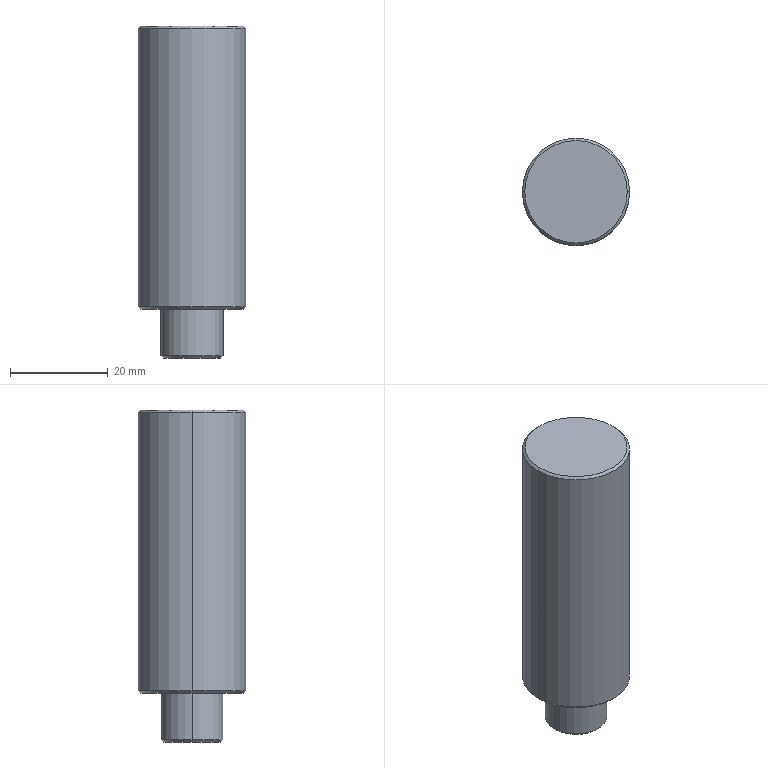Part | SolidWorks | features Chamfer 1, Extrusion 1, ICE 1 | 1 solid | 13 faces | box 22 x 22 x 68 mm | volume 23293 mm3 | cone 6 | cylinder 4 | plane 3 | commonest cylinder face diameters 12.7 x2 22 x2
STEP:
#1=CARTESIAN_POINT('',(-5.85,0.,0.));
#2=VERTEX_POINT('',#1);
#3=CARTESIAN_POINT('',(5.85,0.,0.));
#4=VERTEX_POINT('',#3);
#5=CARTESIAN_POINT('',(0.,0.,0.));
#6=DIRECTION('',(0.,0.,-1.));
#7=DIRECTION('',(1.,0.,0.));
#8=AXIS2_PLACEMENT_3D('',#5,#6,#7);
#9=CIRCLE('',#8,5.85);
#10=EDGE_CURVE('',#2,#4,#9,.T.);
#11=ORIENTED_EDGE('',*,*,#10,.F.);
#12=CARTESIAN_POINT('',(-6.35,0.,0.5));
#13=VERTEX_POINT('',#12);
#14=CARTESIAN_POINT('',(-6.35,0.,0.5));
#15=DIRECTION('',(-0.7071,0.,0.7071));
#16=VECTOR('',#15,1000.);
#17=LINE('',#14,#16);
#18=EDGE_CURVE('',#2,#13,#17,.T.);
#19=ORIENTED_EDGE('',*,*,#18,.T.);
#20=CARTESIAN_POINT('',(6.35,0.,0.5));
#21=VERTEX_POINT('',#20);
#22=CARTESIAN_POINT('',(0.,0.,0.5));
#23=DIRECTION('',(0.,0.,1.));
#24=DIRECTION('',(1.,0.,0.));
#25=AXIS2_PLACEMENT_3D('',#22,#23,#24);
#26=CIRCLE('',#25,6.35);
#27=EDGE_CURVE('',#21,#13,#26,.T.);
#28=ORIENTED_EDGE('',*,*,#27,.F.);
#29=CARTESIAN_POINT('',(6.35,0.,0.5));
#30=DIRECTION('',(0.7071,0.,0.7071));
#31=VECTOR('',#30,1000.);
#32=LINE('',#29,#31);
#33=EDGE_CURVE('',#4,#21,#32,.T.);
#34=ORIENTED_EDGE('',*,*,#33,.F.);
#35=EDGE_LOOP('',(#11,#19,#28,#34));
#36=FACE_OUTER_BOUND('',#35,.T.);
#37=CARTESIAN_POINT('',(0.,0.,0.5));
#38=DIRECTION('',(0.,0.,1.));
#39=DIRECTION('',(1.,0.,0.));
#40=AXIS2_PLACEMENT_3D('',#37,#38,#39);
#41=CONICAL_SURFACE('',#40,6.35,0.7854);
#42=ADVANCED_FACE('',(#36),#41,.T.);
#43=CARTESIAN_POINT('',(10.5,0.,68.));
#44=VERTEX_POINT('',#43);
#45=CARTESIAN_POINT('',(-10.5,0.,68.));
#46=VERTEX_POINT('',#45);
#47=CARTESIAN_POINT('',(0.,0.,68.));
#48=DIRECTION('',(0.,0.,1.));
#49=DIRECTION('',(1.,0.,0.));
#50=AXIS2_PLACEMENT_3D('',#47,#48,#49);
#51=CIRCLE('',#50,10.5);
#52=EDGE_CURVE('',#44,#46,#51,.T.);
#53=ORIENTED_EDGE('',*,*,#52,.F.);
#54=CARTESIAN_POINT('',(11.,0.,67.5));
#55=VERTEX_POINT('',#54);
#56=CARTESIAN_POINT('',(10.5,0.,68.));
#57=DIRECTION('',(0.7071,0.,-0.7071));
#58=VECTOR('',#57,1000.);
#59=LINE('',#56,#58);
#60=EDGE_CURVE('',#44,#55,#59,.T.);
#61=ORIENTED_EDGE('',*,*,#60,.T.);
#62=CARTESIAN_POINT('',(-11.,0.,67.5));
#63=VERTEX_POINT('',#62);
#64=CARTESIAN_POINT('',(0.,0.,67.5));
#65=DIRECTION('',(0.,0.,-1.));
#66=DIRECTION('',(1.,0.,0.));
#67=AXIS2_PLACEMENT_3D('',#64,#65,#66);
#68=CIRCLE('',#67,11.);
#69=EDGE_CURVE('',#63,#55,#68,.T.);
#70=ORIENTED_EDGE('',*,*,#69,.F.);
#71=CARTESIAN_POINT('',(-10.5,0.,68.));
#72=DIRECTION('',(-0.7071,0.,-0.7071));
#73=VECTOR('',#72,1000.);
#74=LINE('',#71,#73);
#75=EDGE_CURVE('',#46,#63,#74,.T.);
#76=ORIENTED_EDGE('',*,*,#75,.F.);
#77=EDGE_LOOP('',(#53,#61,#70,#76));
#78=FACE_OUTER_BOUND('',#77,.T.);
#79=CARTESIAN_POINT('',(0.,0.,68.));
#80=DIRECTION('',(0.,0.,-1.));
#81=DIRECTION('',(-1.,0.,0.));
#82=AXIS2_PLACEMENT_3D('',#79,#80,#81);
#83=CONICAL_SURFACE('',#82,10.5,0.7854);
#84=ADVANCED_FACE('',(#78),#83,.T.);
#85=CARTESIAN_POINT('',(-10.5,0.,10.));
#86=VERTEX_POINT('',#85);
#87=CARTESIAN_POINT('',(10.5,0.,10.));
#88=VERTEX_POINT('',#87);
#89=CARTESIAN_POINT('',(0.,0.,10.));
#90=DIRECTION('',(0.,0.,-1.));
#91=DIRECTION('',(1.,0.,0.));
#92=AXIS2_PLACEMENT_3D('',#89,#90,#91);
#93=CIRCLE('',#92,10.5);
#94=EDGE_CURVE('',#86,#88,#93,.T.);
#95=ORIENTED_EDGE('',*,*,#94,.F.);
#96=CARTESIAN_POINT('',(-11.,0.,10.5));
#97=VERTEX_POINT('',#96);
#98=CARTESIAN_POINT('',(-11.,0.,10.5));
#99=DIRECTION('',(-0.7071,0.,0.7071));
#100=VECTOR('',#99,1000.);
#101=LINE('',#98,#100);
#102=EDGE_CURVE('',#86,#97,#101,.T.);
#103=ORIENTED_EDGE('',*,*,#102,.T.);
#104=CARTESIAN_POINT('',(11.,0.,10.5));
#105=VERTEX_POINT('',#104);
#106=CARTESIAN_POINT('',(0.,0.,10.5));
#107=DIRECTION('',(0.,0.,1.));
#108=DIRECTION('',(1.,0.,0.));
#109=AXIS2_PLACEMENT_3D('',#106,#107,#108);
#110=CIRCLE('',#109,11.);
#111=EDGE_CURVE('',#105,#97,#110,.T.);
#112=ORIENTED_EDGE('',*,*,#111,.F.);
#113=CARTESIAN_POINT('',(11.,0.,10.5));
#114=DIRECTION('',(0.7071,0.,0.7071));
#115=VECTOR('',#114,1000.);
#116=LINE('',#113,#115);
#117=EDGE_CURVE('',#88,#105,#116,.T.);
#118=ORIENTED_EDGE('',*,*,#117,.F.);
#119=EDGE_LOOP('',(#95,#103,#112,#118));
#120=FACE_OUTER_BOUND('',#119,.T.);
#121=CARTESIAN_POINT('',(0.,0.,10.5));
#122=DIRECTION('',(0.,0.,1.));
#123=DIRECTION('',(1.,0.,0.));
#124=AXIS2_PLACEMENT_3D('',#121,#122,#123);
#125=CONICAL_SURFACE('',#124,11.,0.7854);
#126=ADVANCED_FACE('',(#120),#125,.T.);
#127=ORIENTED_EDGE('',*,*,#69,.T.);
#128=CARTESIAN_POINT('',(11.,0.,68.));
#129=DIRECTION('',(0.,0.,-1.));
#130=VECTOR('',#129,1000.);
#131=LINE('',#128,#130);
#132=EDGE_CURVE('',#55,#105,#131,.T.);
#133=ORIENTED_EDGE('',*,*,#132,.T.);
#134=ORIENTED_EDGE('',*,*,#111,.T.);
#135=CARTESIAN_POINT('',(-11.,0.,68.));
#136=DIRECTION('',(0.,0.,-1.));
#137=VECTOR('',#136,1000.);
#138=LINE('',#135,#137);
#139=EDGE_CURVE('',#63,#97,#138,.T.);
#140=ORIENTED_EDGE('',*,*,#139,.F.);
#141=EDGE_LOOP('',(#127,#133,#134,#140));
#142=FACE_OUTER_BOUND('',#141,.T.);
#143=CARTESIAN_POINT('',(0.,0.,68.));
#144=DIRECTION('',(0.,0.,-1.));
#145=DIRECTION('',(-1.,0.,0.));
#146=AXIS2_PLACEMENT_3D('',#143,#144,#145);
#147=CYLINDRICAL_SURFACE('',#146,11.);
#148=ADVANCED_FACE('',(#142),#147,.T.);
#149=CARTESIAN_POINT('',(6.35,0.,10.));
#150=VERTEX_POINT('',#149);
#151=CARTESIAN_POINT('',(-6.35,0.,10.));
#152=VERTEX_POINT('',#151);
#153=CARTESIAN_POINT('',(0.,0.,10.));
#154=DIRECTION('',(0.,0.,1.));
#155=DIRECTION('',(1.,0.,0.));
#156=AXIS2_PLACEMENT_3D('',#153,#154,#155);
#157=CIRCLE('',#156,6.35);
#158=EDGE_CURVE('',#150,#152,#157,.T.);
#159=ORIENTED_EDGE('',*,*,#158,.F.);
#160=CARTESIAN_POINT('',(6.35,0.,10.));
#161=DIRECTION('',(0.,0.,-1.));
#162=VECTOR('',#161,1000.);
#163=LINE('',#160,#162);
#164=EDGE_CURVE('',#150,#21,#163,.T.);
#165=ORIENTED_EDGE('',*,*,#164,.T.);
#166=ORIENTED_EDGE('',*,*,#27,.T.);
#167=CARTESIAN_POINT('',(-6.35,0.,10.));
#168=DIRECTION('',(0.,0.,-1.));
#169=VECTOR('',#168,1000.);
#170=LINE('',#167,#169);
#171=EDGE_CURVE('',#152,#13,#170,.T.);
#172=ORIENTED_EDGE('',*,*,#171,.F.);
#173=EDGE_LOOP('',(#159,#165,#166,#172));
#174=FACE_OUTER_BOUND('',#173,.T.);
#175=CARTESIAN_POINT('',(0.,0.,10.));
#176=DIRECTION('',(0.,0.,-1.));
#177=DIRECTION('',(-1.,0.,0.));
#178=AXIS2_PLACEMENT_3D('',#175,#176,#177);
#179=CYLINDRICAL_SURFACE('',#178,6.35);
#180=ADVANCED_FACE('',(#174),#179,.T.);
#181=ORIENTED_EDGE('',*,*,#164,.F.);
#182=CARTESIAN_POINT('',(0.,0.,10.));
#183=DIRECTION('',(0.,0.,1.));
#184=DIRECTION('',(1.,0.,0.));
#185=AXIS2_PLACEMENT_3D('',#182,#183,#184);
#186=CIRCLE('',#185,6.35);
#187=EDGE_CURVE('',#152,#150,#186,.T.);
#188=ORIENTED_EDGE('',*,*,#187,.F.);
#189=ORIENTED_EDGE('',*,*,#171,.T.);
#190=CARTESIAN_POINT('',(0.,0.,0.5));
#191=DIRECTION('',(0.,0.,1.));
#192=DIRECTION('',(1.,0.,0.));
#193=AXIS2_PLACEMENT_3D('',#190,#191,#192);
#194=CIRCLE('',#193,6.35);
#195=EDGE_CURVE('',#13,#21,#194,.T.);
#196=ORIENTED_EDGE('',*,*,#195,.T.);
#197=EDGE_LOOP('',(#181,#188,#189,#196));
#198=FACE_OUTER_BOUND('',#197,.T.);
#199=CARTESIAN_POINT('',(0.,0.,10.));
#200=DIRECTION('',(0.,0.,-1.));
#201=DIRECTION('',(-1.,0.,0.));
#202=AXIS2_PLACEMENT_3D('',#199,#200,#201);
#203=CYLINDRICAL_SURFACE('',#202,6.35);
#204=ADVANCED_FACE('',(#198),#203,.T.);
#205=CARTESIAN_POINT('',(0.,0.,0.));
#206=DIRECTION('',(0.,0.,-1.));
#207=DIRECTION('',(1.,0.,0.));
#208=AXIS2_PLACEMENT_3D('',#205,#206,#207);
#209=CIRCLE('',#208,5.85);
#210=EDGE_CURVE('',#4,#2,#209,.T.);
#211=ORIENTED_EDGE('',*,*,#210,.T.);
#212=ORIENTED_EDGE('',*,*,#10,.T.);
#213=EDGE_LOOP('',(#211,#212));
#214=FACE_OUTER_BOUND('',#213,.T.);
#215=CARTESIAN_POINT('',(0.,0.,0.));
#216=DIRECTION('',(0.,0.,1.));
#217=DIRECTION('',(1.,0.,0.));
#218=AXIS2_PLACEMENT_3D('',#215,#216,#217);
#219=PLANE('',#218);
#220=ADVANCED_FACE('',(#214),#219,.F.);
#221=ORIENTED_EDGE('',*,*,#132,.F.);
#222=CARTESIAN_POINT('',(0.,0.,67.5));
#223=DIRECTION('',(0.,0.,-1.));
#224=DIRECTION('',(1.,0.,0.));
#225=AXIS2_PLACEMENT_3D('',#222,#223,#224);
#226=CIRCLE('',#225,11.);
#227=EDGE_CURVE('',#55,#63,#226,.T.);
#228=ORIENTED_EDGE('',*,*,#227,.T.);
#229=ORIENTED_EDGE('',*,*,#139,.T.);
#230=CARTESIAN_POINT('',(0.,0.,10.5));
#231=DIRECTION('',(0.,0.,1.));
#232=DIRECTION('',(1.,0.,0.));
#233=AXIS2_PLACEMENT_3D('',#230,#231,#232);
#234=CIRCLE('',#233,11.);
#235=EDGE_CURVE('',#97,#105,#234,.T.);
#236=ORIENTED_EDGE('',*,*,#235,.T.);
#237=EDGE_LOOP('',(#221,#228,#229,#236));
#238=FACE_OUTER_BOUND('',#237,.T.);
#239=CARTESIAN_POINT('',(0.,0.,68.));
#240=DIRECTION('',(0.,0.,-1.));
#241=DIRECTION('',(-1.,0.,0.));
#242=AXIS2_PLACEMENT_3D('',#239,#240,#241);
#243=CYLINDRICAL_SURFACE('',#242,11.);
#244=ADVANCED_FACE('',(#238),#243,.T.);
#245=CARTESIAN_POINT('',(0.,0.,68.));
#246=DIRECTION('',(0.,0.,1.));
#247=DIRECTION('',(1.,0.,0.));
#248=AXIS2_PLACEMENT_3D('',#245,#246,#247);
#249=CIRCLE('',#248,10.5);
#250=EDGE_CURVE('',#46,#44,#249,.T.);
#251=ORIENTED_EDGE('',*,*,#250,.T.);
#252=ORIENTED_EDGE('',*,*,#52,.T.);
#253=EDGE_LOOP('',(#251,#252));
#254=FACE_OUTER_BOUND('',#253,.T.);
#255=CARTESIAN_POINT('',(0.,0.,68.));
#256=DIRECTION('',(0.,0.,1.));
#257=DIRECTION('',(1.,0.,0.));
#258=AXIS2_PLACEMENT_3D('',#255,#256,#257);
#259=PLANE('',#258);
#260=ADVANCED_FACE('',(#254),#259,.T.);
#261=CARTESIAN_POINT('',(0.,0.,10.));
#262=DIRECTION('',(0.,0.,-1.));
#263=DIRECTION('',(1.,0.,0.));
#264=AXIS2_PLACEMENT_3D('',#261,#262,#263);
#265=CIRCLE('',#264,10.5);
#266=EDGE_CURVE('',#88,#86,#265,.T.);
#267=ORIENTED_EDGE('',*,*,#266,.T.);
#268=ORIENTED_EDGE('',*,*,#94,.T.);
#269=EDGE_LOOP('',(#267,#268));
#270=FACE_OUTER_BOUND('',#269,.T.);
#271=ORIENTED_EDGE('',*,*,#187,.T.);
#272=ORIENTED_EDGE('',*,*,#158,.T.);
#273=EDGE_LOOP('',(#271,#272));
#274=FACE_BOUND('',#273,.T.);
#275=CARTESIAN_POINT('',(0.,0.,10.));
#276=DIRECTION('',(0.,0.,1.));
#277=DIRECTION('',(1.,0.,0.));
#278=AXIS2_PLACEMENT_3D('',#275,#276,#277);
#279=PLANE('',#278);
#280=ADVANCED_FACE('',(#270,#274),#279,.F.);
#281=ORIENTED_EDGE('',*,*,#102,.F.);
#282=ORIENTED_EDGE('',*,*,#266,.F.);
#283=ORIENTED_EDGE('',*,*,#117,.T.);
#284=ORIENTED_EDGE('',*,*,#235,.F.);
#285=EDGE_LOOP('',(#281,#282,#283,#284));
#286=FACE_OUTER_BOUND('',#285,.T.);
#287=CARTESIAN_POINT('',(0.,0.,10.5));
#288=DIRECTION('',(0.,0.,1.));
#289=DIRECTION('',(1.,0.,0.));
#290=AXIS2_PLACEMENT_3D('',#287,#288,#289);
#291=CONICAL_SURFACE('',#290,11.,0.7854);
#292=ADVANCED_FACE('',(#286),#291,.T.);
#293=ORIENTED_EDGE('',*,*,#60,.F.);
#294=ORIENTED_EDGE('',*,*,#250,.F.);
#295=ORIENTED_EDGE('',*,*,#75,.T.);
#296=ORIENTED_EDGE('',*,*,#227,.F.);
#297=EDGE_LOOP('',(#293,#294,#295,#296));
#298=FACE_OUTER_BOUND('',#297,.T.);
#299=CARTESIAN_POINT('',(0.,0.,68.));
#300=DIRECTION('',(0.,0.,-1.));
#301=DIRECTION('',(-1.,0.,0.));
#302=AXIS2_PLACEMENT_3D('',#299,#300,#301);
#303=CONICAL_SURFACE('',#302,10.5,0.7854);
#304=ADVANCED_FACE('',(#298),#303,.T.);
#305=ORIENTED_EDGE('',*,*,#18,.F.);
#306=ORIENTED_EDGE('',*,*,#210,.F.);
#307=ORIENTED_EDGE('',*,*,#33,.T.);
#308=ORIENTED_EDGE('',*,*,#195,.F.);
#309=EDGE_LOOP('',(#305,#306,#307,#308));
#310=FACE_OUTER_BOUND('',#309,.T.);
#311=CARTESIAN_POINT('',(0.,0.,0.5));
#312=DIRECTION('',(0.,0.,1.));
#313=DIRECTION('',(1.,0.,0.));
#314=AXIS2_PLACEMENT_3D('',#311,#312,#313);
#315=CONICAL_SURFACE('',#314,6.35,0.7854);
#316=ADVANCED_FACE('',(#310),#315,.T.);
#317=CLOSED_SHELL('',(#42,#84,#126,#148,#180,#204,#220,#244,#260,#280,#292,#304,#316));
#318=MANIFOLD_SOLID_BREP('',#317);
#319=CARTESIAN_POINT('',(0.,0.,0.));
#320=DIRECTION('',(0.,0.,1.));
#321=DIRECTION('',(1.,0.,0.));
#322=AXIS2_PLACEMENT_3D('',#319,#320,#321);
#323=(LENGTH_UNIT()NAMED_UNIT(*)SI_UNIT(.MILLI.,.METRE.));
#324=UNCERTAINTY_MEASURE_WITH_UNIT(LENGTH_MEASURE(0.00001),#323,'','');
#325=(NAMED_UNIT(*)PLANE_ANGLE_UNIT()SI_UNIT($,.RADIAN.));
#326=(NAMED_UNIT(*)SI_UNIT($,.STERADIAN.)SOLID_ANGLE_UNIT());
#327=(GEOMETRIC_REPRESENTATION_CONTEXT(3)GLOBAL_UNCERTAINTY_ASSIGNED_CONTEXT((#324))GLOBAL_UNIT_ASSIGNED_CONTEXT((#323,#325,#326))REPRESENTATION_CONTEXT('',''));
#328=ADVANCED_BREP_SHAPE_REPRESENTATION('',(#318,#322),#327);